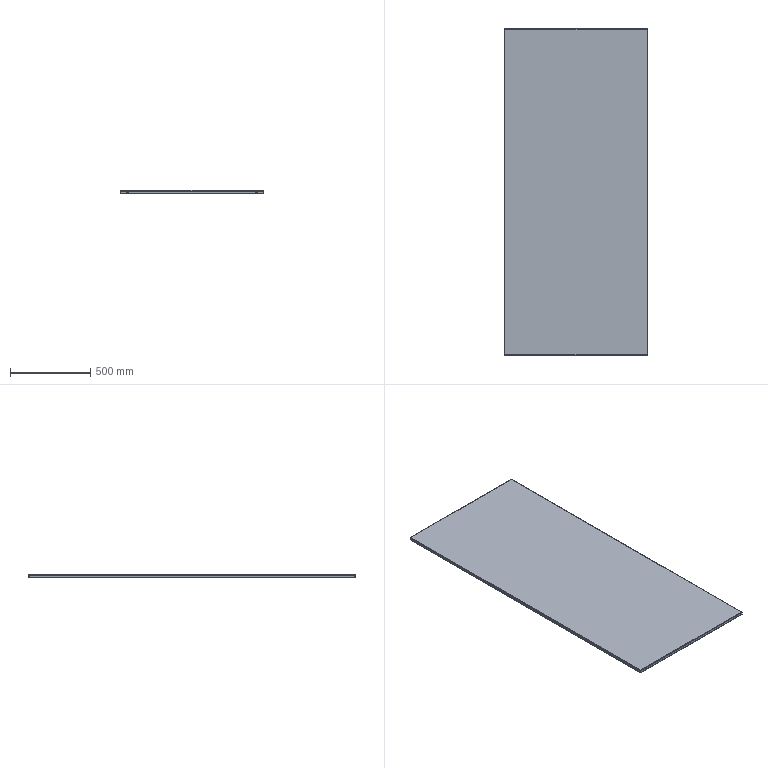Part | STEP file | 750038411 | 1 solid | 66 faces | box 896 x 2036 x 20 mm | volume 4018739 mm3 | plane 46 | cylinder 20 | commonest cylinder face diameters 2 x4 4 x4 6 x4 8 x4 9 x4